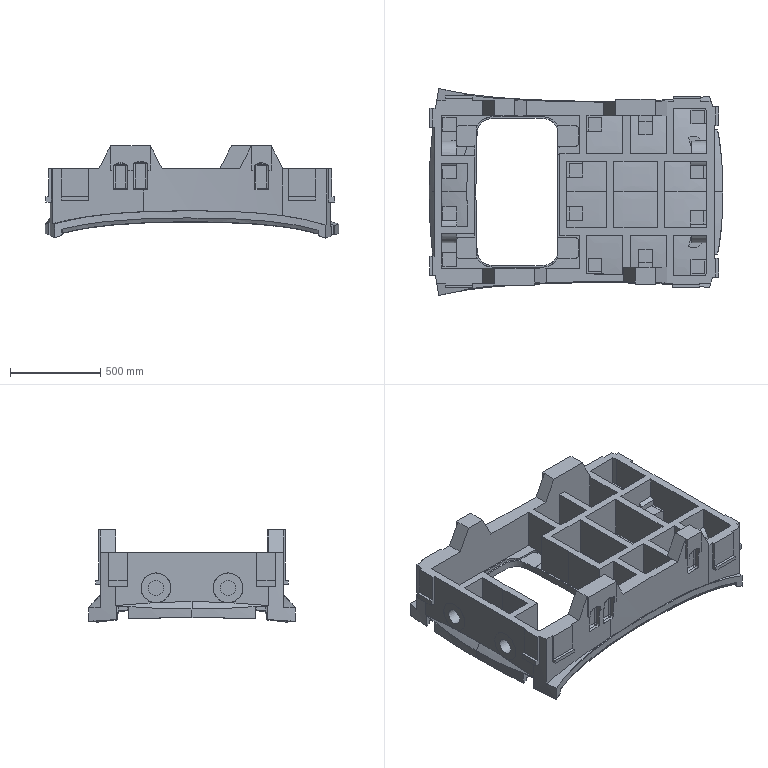Part | NX | features MAIN_BODY 2 | 1 solid | 848 faces | box 1628 x 1146 x 512.793 mm | volume 199985710 mm3 | plane 385 | spline 287 | cylinder 148 | torus 12 | sphere 12 | cone 4 | commonest cylinder face diameters 20 x46 165 x18 80 x16 70 x12 10 x10 100 x10